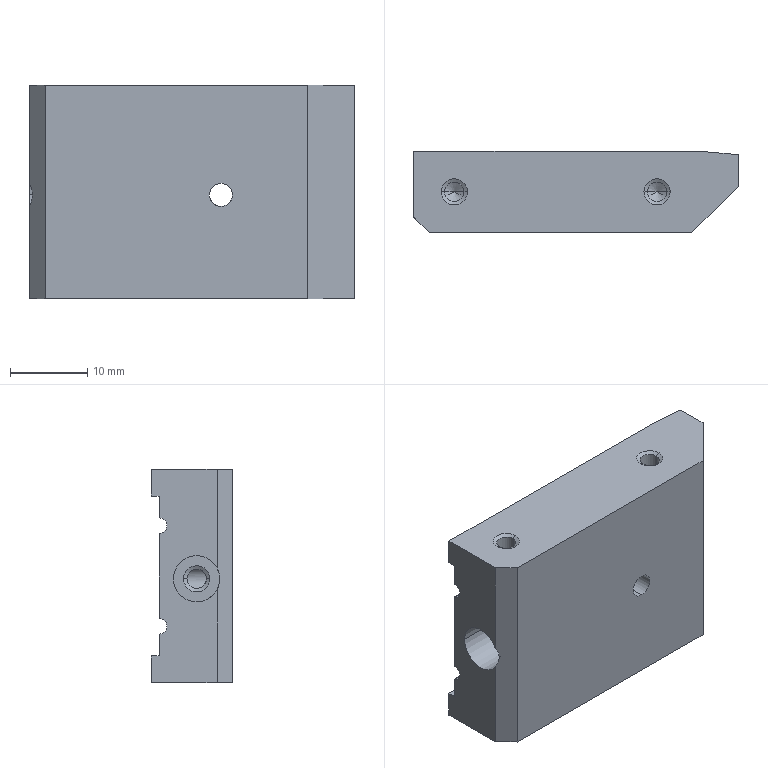Part | NX | 1 solid | 67 faces | box 42 x 10.5 x 27.6 mm | volume 10010 mm3 | cylinder 30 | cone 20 | plane 17 | commonest cylinder face diameters 2.5 x18 0.4 x4 2 x4 3 x2 6 x2